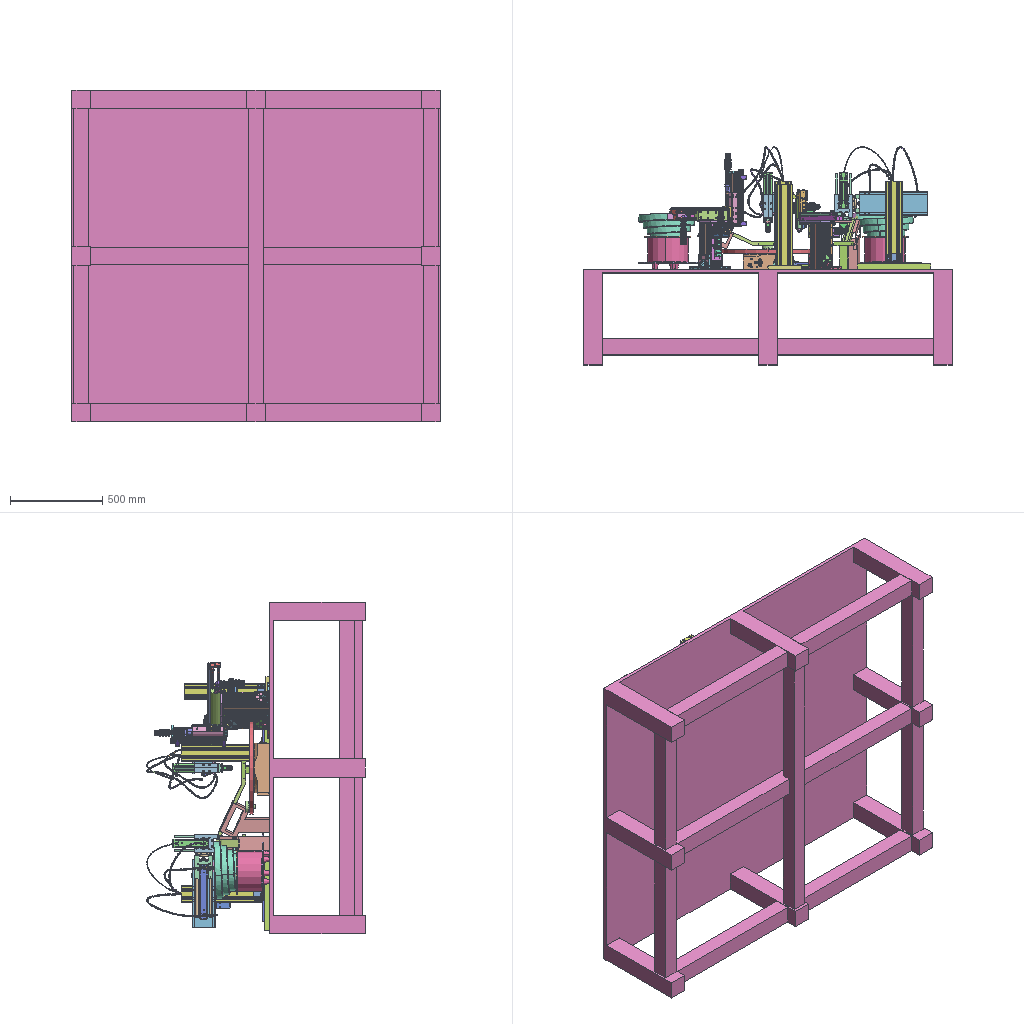Assembly | STEP file | 117 different items | 203 placed | box 2000 x 1188 x 1800 mm
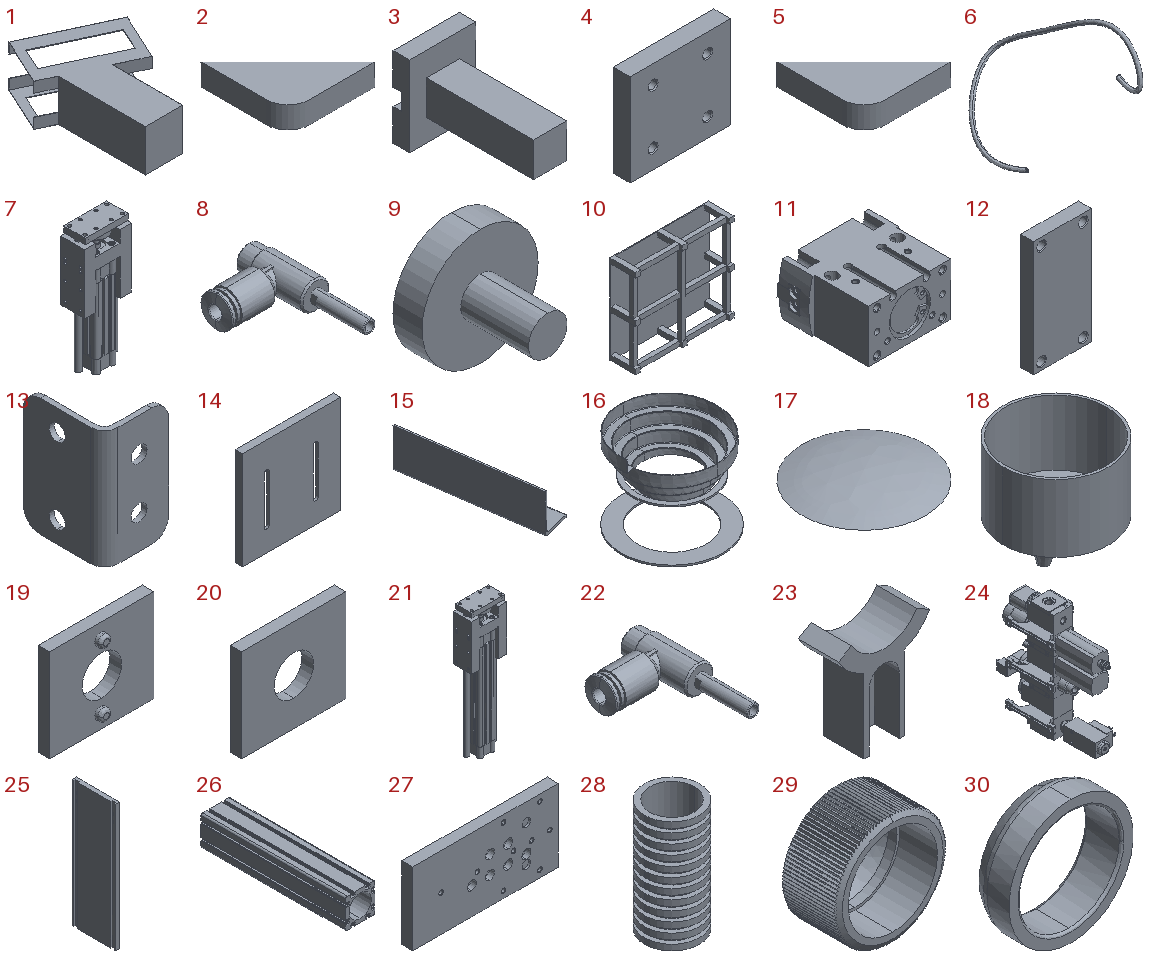Parts list (item | name | quantity | parent item | size | volume):
1 | Part3_4 | x2 | in BOBBIN PRESSING MACHINE | 195.46 x 270.819 x 80 mm | 83841 mm3
2 | Part9_5 | x6 | in BOBBIN PRESSING MACHINE | 20 x 20 x 5 mm | 973.175 mm3
3 | Part1_4 | x2 | in BOBBIN PRESSING MACHINE | 80 x 149.9 x 97 mm | 359263 mm3
4 | 555_4 | x2 | in BOBBIN PRESSING MACHINE | 60 x 10 x 54.9 mm | 31707 mm3
5 | Part8_5 | x6 | in BOBBIN PRESSING MACHINE | 20 x 20 x 5 mm | 973.175 mm3
6 | 332_4 | x2 | in BOBBIN PRESSING MACHINE | 176.185 x 279.344 x 194.737 mm | 23581 mm3
7 | 535411 DNCI-32-100-P-A-FENG-MS---(asm_0_)(control position cylinder 100)_5 | x2 | in BOBBIN PRESSING MACHINE | 97 x 50 x 265 mm | 701103 mm3
8 | 1_11 | x4 | in BOBBIN PRESSING MACHINE | 24.75 x 38 x 10 mm | 2280 mm3
9 | Part5_1 | x1 | in BOBBIN PRESSING MACHINE | 60 x 50 x 60 mm | 49793 mm3
10 | 223_4 | x1 | in BOBBIN PRESSING MACHINE | 2000 x 520 x 1800 mm | 184958483 mm3
11 | 535861 HGPT-20-A---(asm_0)_5 | x2 | in BOBBIN PRESSING MACHINE | 50 x 46 x 28 mm | 52148 mm3
12 | spacer_5 | x2 | in BOBBIN PRESSING MACHINE | 45 x 10 x 90 mm | 39110 mm3
13 | Part6_5 | x6 | in BOBBIN PRESSING MACHINE | 38 x 48 x 70 mm | 15736 mm3
14 | leg control03_5 | x2 | in BOBBIN PRESSING MACHINE | 400 x 30 x 400 mm | 2067797 mm3
15 | 444_4 | x2 | in bowel feeder_4 | 42.378 x 132.163 x 37.433 mm | 15585 mm3
16 | 222_4 | x2 | in bowel feeder_4 | 322.673 x 320.624 x 270.209 mm | 556791 mm3
17 | 111_4 | x2 | in bowel feeder_4 | 185.942 x 185.942 x 13.599 mm | 185950 mm3
18 | 333_4 | x2 | in bowel feeder_4 | 220 x 220 x 180 mm | 733955 mm3
19 | leg control01_5 | x2 | in BOBBIN PRESSING MACHINE | 180 x 30 x 160 mm | 509091 mm3
20 | Part10_5 | x1 | in BOBBIN PRESSING MACHINE | 180 x 20 x 160 mm | 503407 mm3
21 | 535411 DNCI-32-200-P-A-FENG-MS---(asm_0_)(control position cylinder with guide)_5 | x2 | in BOBBIN PRESSING MACHINE | 97 x 50 x 365 mm | 831843 mm3
22 | 1_10 | x4 | in BOBBIN PRESSING MACHINE | 24.75 x 38 x 10 mm | 2280 mm3
23 | jaw_5 | x4 | in BOBBIN PRESSING MACHINE | 18.187 x 8 x 20.75 mm | 920.185 mm3
24 | 542315 MSB4-1_4_C3J4M1D1A1F3-WP_5 | x1 | in BOBBIN PRESSING MACHINE | 85 x 221.2 x 244.7 mm | 1168039 mm3
25 | Part7_5 | x2 | in BOBBIN PRESSING MACHINE | 12 x 127 x 370 mm | 526068 mm3
26 | leg01_5 | x3 | in BOBBIN PRESSING MACHINE | 90 x 440 x 90 mm | 1490360 mm3
27 | 00684281_ADAPTERPLATTE_HMVY-1 | x1 | in 00539968_EZT_VERBINDUNGS-BS_HMVY-1 | 160 x 12 x 80 mm | 147813 mm3
28 | P0177567_EZT_SCHUTZSCHLAUCH_MKR-23-PG-21.1 | x1 | in HMI... | 28.5 x 28.5 x 58 mm | 8821 mm3
29 | 00649789_MUTTER_RAENDEL_MKRT-23-16.5 | x2 | in 00194321_EZT_SCHUTZSCHL.VERB_MKRT-23-16.5.1 | 35.488 x 19 x 35.5 mm | 6985 mm3
30 | 00399797_RING_ELASTOMER_MKRT-23-16.5 | x2 | in 00194321_EZT_SCHUTZSCHL.VERB_MKRT-23-16.5.1 | 26.7 x 8 x 26.7 mm | 1330 mm3
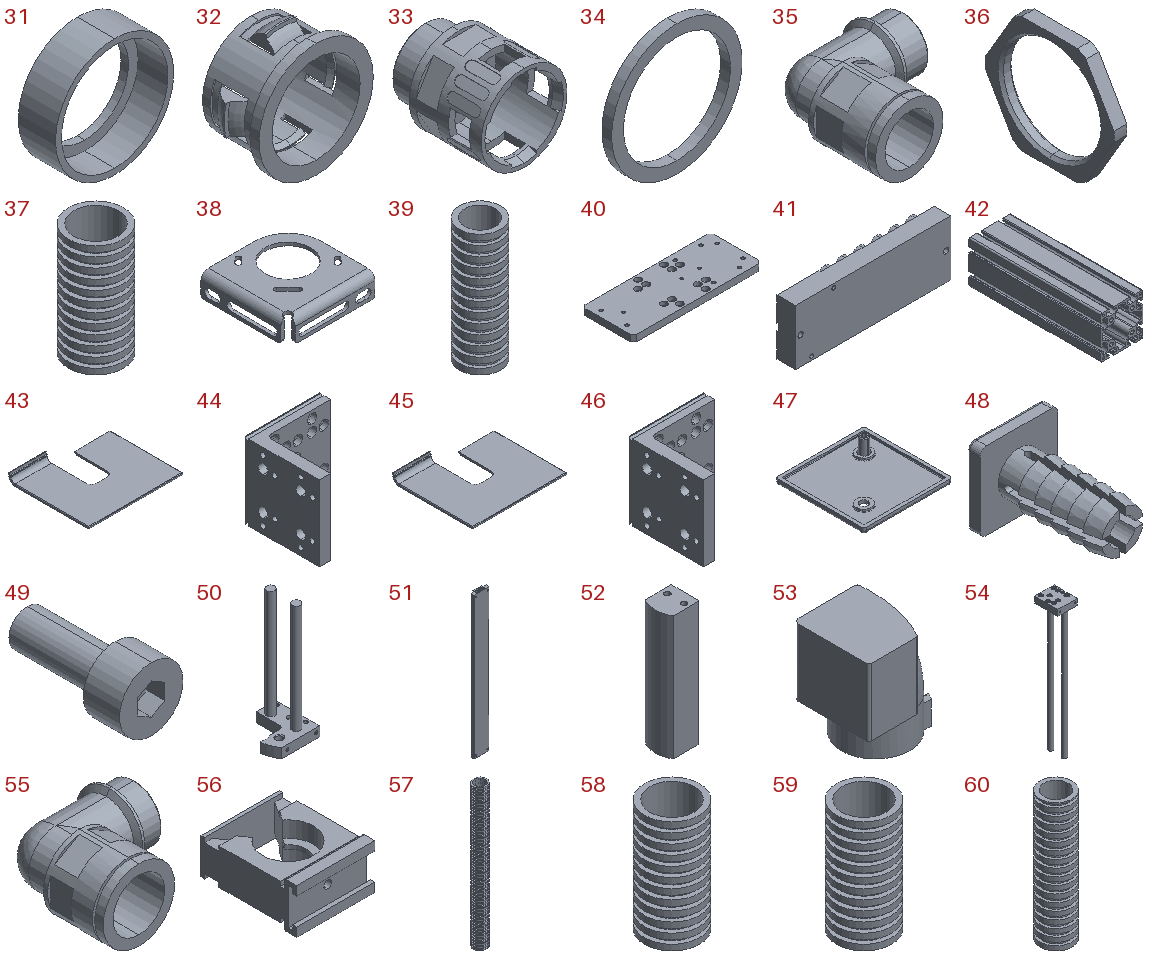31 | P2858E27_RING_DICHT | x4 | in 00177572_SCHUTZSCHL.VERS_MKRV-23-PG-21, 00177572_SCHUTZSCHL.VERS_MKRV-23-PG-21.1 | 31.6 x 10 x 31.6 mm | 1879 mm3
32 | P2858E25_EINSATZ_VERSCH. | x4 | in 00177572_SCHUTZSCHL.VERS_MKRV-23-PG-21, 00177572_SCHUTZSCHL.VERS_MKRV-23-PG-21.1 | 37 x 21 x 37 mm | 4042 mm3
33 | PN_0001 part X2_00DC_X0 throw | x4 | in 00177572_SCHUTZSCHL.VERS_MKRV-23-PG-21, 00177572_SCHUTZSCHL.VERS_MKRV-23-PG-21.1 | 37 x 43 x 37 mm | 10248 mm3
34 | 00649788_SCHEIBE_MKRT-23-16.5 | x2 | in 00194321_EZT_SCHUTZSCHL.VERB_MKRT-23-16.5.1 | 26.5 x 2 x 26.5 mm | 360.007 mm3
35 | 00177576_EZT_L-SCH.SCHL.VER._MKRL-16.5-PG-16 | x1 | in HMI... | 50.5 x 51.75 x 29.5 mm | 15308 mm3
36 | 00373407_MUTTER_M_PG_21_DIN_46320-MS | x3 | in 00177599_EZT_GEGENMUTTER_MKM-PG-21.1 | 3.5 x 35.5 x 32 mm | 1055 mm3
37 | P0177567_EZT_SCHUTZSCHLAUCH_MKR-23-PG-21.2 | x1 | in HMI... | 28.5 x 28.5 x 58 mm | 8821 mm3
38 | 00396465_ADAPTER_HMZAS-PG21 | x3 | in 00193124_EZT_ADAPTERPLATTE_HMZAS-PG-21.1 | 54.5 x 54.5 x 14 mm | 5523 mm3
39 | P0177566_EZT_SCHUTZSCHLAUCH_MKR-16.5-PG-16 | x1 | in HMI... | 21.2 x 21.2 x 63 mm | 7207 mm3
40 | 00398494_EZT_ADAPTERPLATTE_HMZV-1 | x1 | in HMZV-1 | 200 x 80 x 10 mm | 151646 mm3
41 | PRODUCT_NAME_42 | x1 | in 177670_MPV-E_A12-M8 | 126 x 19.5 x 45 mm | 83234 mm3
42 | 00175958_EZT_PROFILSAEULE_HMBS-80.80-250-.1 | x1 | in HMBS-1 | 80 x 250 x 80 mm | 517689 mm3
43 | 00371716_ABDECKKAPPE_HMB-....2 | x2 | in 00175967_EZT_VERBINDUNGS-BS_HMBV-ND.1 | 79.8 x 67.8 x 10.238 mm | 5792 mm3
44 | 00363089_WINKEL_HMB-..._1 | x1 | in 00175967_EZT_VERBINDUNGS-BS_HMBV-ND.1 | 80 x 80 x 80 mm | 130537 mm3
45 | 00371716_ABDECKKAPPE_HMB-....1 | x4 | in 00175951_EZT_GRUND-BS_HMBF-DB.1 | 79.8 x 67.8 x 10.238 mm | 5792 mm3
46 | 00363089_WINKEL_HMB-... | x2 | in 00175951_EZT_GRUND-BS_HMBF-DB.1 | 80 x 80 x 80 mm | 130537 mm3
47 | 00369089_KAPPE_ABDECK_IPM-AN-8-80X80 | x1 | in 00175965_ABDECKKAPPE_HMBSA-80_80.1 | 80 x 80 x 18 mm | 20980 mm3
48 | 00369095_STOPFEN_BEFEST._IPM-AB-8-SW | x1 | in 00175965_ABDECKKAPPE_HMBSA-80_80.1 | 12 x 18.5 x 12 mm | 599.689 mm3
49 | - | x4 | in 191182_HMPL-16-160-AI-VP-2A2 | 7 x 14 x 7 mm | 263.372 mm3
50 | - | x1 | in 191182_HMPL-16-160-AI-VP-2A2 | 54.828 x 55 x 147.5 mm | 42895 mm3
51 | P193368_BVP_HMPL_16_160 | x1 | in 191182_HMPL-16-160-AI-VP-2A2 | 45 x 14 x 426.6 mm | 169280 mm3
52 | - | x1 | in 191182_HMPL-16-160-AI-VP-2A2 | 56.5 x 53 x 234 mm | 627252 mm3
53 | P393261_cap_HMPL_16 | x1 | in 191182_HMPL-16-160-AI-VP-2A2 | 36.5 x 32.1 x 42.5 mm | 33239 mm3
54 | - | x1 | in 191182_HMPL-16-160-AI-VP-2A2 | 45 x 54 x 319 mm | 75910 mm3
55 | 00177577_EZT_L-SCH.SCHL.VER._MKRL-23-PG-21.1 | x1 | in HMI..._1 | 59.35 x 59.85 x 37 mm | 23850 mm3
56 | 00192290_EZT_KLEMMSCHELLE_MKRS-23-B.2 | x2 | in HMI..._1 | 43.5 x 53.5 x 25 mm | 24720 mm3
57 | P0177567_EZT_SCHUTZSCHLAUCH_MKR-23-PG-21.2_1 | x1 | in HMI..._1 | 28.5 x 28.5 x 303 mm | 45141 mm3
58 | P0177567_EZT_SCHUTZSCHLAUCH_MKR-23-PG-21.1_1 | x1 | in HMI..._1 | 28.5 x 28.5 x 58 mm | 8821 mm3
59 | P0177567_EZT_SCHUTZSCHLAUCH_MKR-23-PG-21.3 | x1 | in HMI..._1 | 28.5 x 28.5 x 58 mm | 8821 mm3
60 | P0177566_EZT_SCHUTZSCHLAUCH_MKR-16.5-PG-16_1 | x1 | in HMI..._1 | 21.2 x 21.2 x 85.851 mm | 9693 mm3
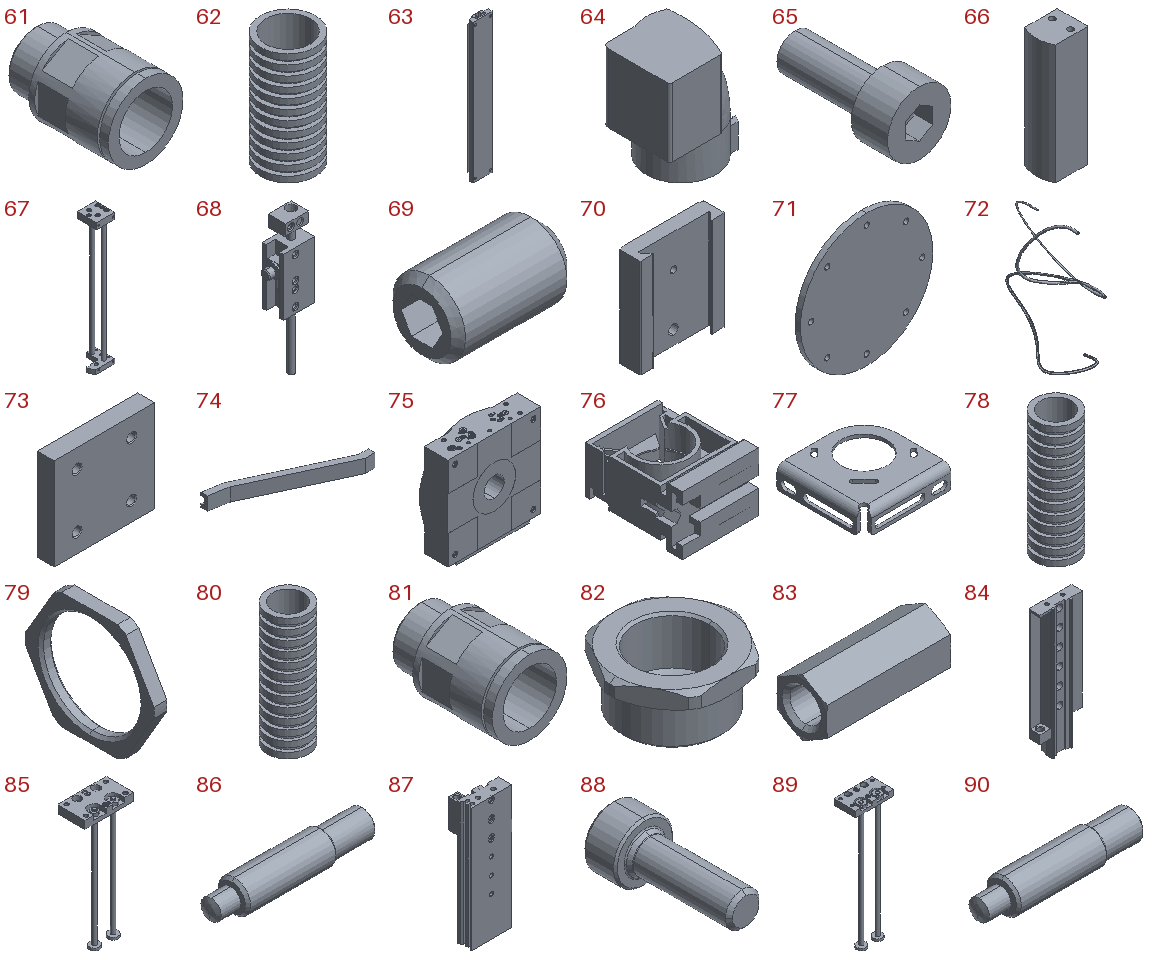61 | 00177571_EZT_SCHUTZSCHL.VERS_MKRV-16.5-PG-16.1 | x1 | in HMI..._1 | 29.5 x 43.5 x 29.5 mm | 11816 mm3
62 | P0177567_EZT_SCHUTZSCHLAUCH_MKR-23-PG-21.4 | x1 | in HMI..._1 | 28.5 x 28.5 x 58 mm | 8821 mm3
63 | P193372_BVP_HMPL_12_100 | x1 | in 191181_HMPL-12-100-AI-VP-KP-2A2 | 42 x 14 x 301.6 mm | 121442 mm3
64 | P393295_cap_HMPL_12 | x1 | in 191181_HMPL-12-100-AI-VP-KP-2A2 | 36.5 x 29.25 x 42.5 mm | 30561 mm3
65 | - | x4 | in 191181_HMPL-12-100-AI-VP-KP-2A2 | 7 x 14 x 7 mm | 263.372 mm3
66 | - | x1 | in 191181_HMPL-12-100-AI-VP-KP-2A2 | 51.8 x 44 x 171 mm | 352812 mm3
67 | - | x1 | in 191181_HMPL-12-100-AI-VP-KP-2A2 | 50.109 x 46 x 302 mm | 63535 mm3
68 | 00193112_FESTSTELLEINH._BKP-HMPL-12-80.100 | x1 | in 191181_HMPL-12-100-AI-VP-KP-2A2 | 52.1 x 29 x 190 mm | 85928 mm3
69 | 00245858_Gewinsestift | x2 | in 00193126_EZT_KLEMMELEMENT_HMPL-..-...2 | 10 x 6 x 6 mm | 243.919 mm3
70 | 00382584_HALTER_SCHWALB._HMPL-..-.. | x2 | in 00193126_EZT_KLEMMELEMENT_HMPL-..-...2 | 42 x 11 x 49 mm | 15212 mm3
71 | 113_4 | x1 | in BOBBIN PRESSING MACHINE | 500 x 20 x 500 mm | 3876725 mm3
72 | Part4_2 | x2 | in BOBBIN PRESSING MACHINE | - | -
73 | 442_4 | x2 | in BOBBIN PRESSING MACHINE | 60 x 10 x 54.9 mm | 31707 mm3
74 | Part2_4 | x2 | in BOBBIN PRESSING MACHINE | 368.104 x 160 x 40 mm | 215115 mm3
75 | 163302 DNC-32-200-P-A-V5---(asm_200)(index)_5 | x1 | in BOBBIN PRESSING MACHINE | 270 x 89 x 286.6 mm | 5960531 mm3
76 | 00192289_KLEMMSCHELLE_MKRS-16.5-B.1 | x1 | in HMI..._3 | 36.5 x 41.5 x 25 mm | 11692 mm3
77 | 00396465_ADAPTER_HMZAS-PG21_3 | x1 | in 00193124_EZT_ADAPTERPLATTE_HMZAS-PG-21.1_2 | 54.5 x 54.5 x 14 mm | 5523 mm3
78 | P0177566_EZT_SCHUTZSCHLAUCH_MKR-16.5-PG-16.2 | x1 | in HMI..._3 | 21.2 x 21.2 x 63 mm | 7207 mm3
79 | 00373407_MUTTER_M_PG_21_DIN_46320-MS_3 | x1 | in 00177599_EZT_GEGENMUTTER_MKM-PG-21.1_2 | 3.5 x 35.5 x 32 mm | 1055 mm3
80 | P0177566_EZT_SCHUTZSCHLAUCH_MKR-16.5-PG-16.1 | x1 | in HMI..._3 | 21.2 x 21.2 x 63 mm | 7207 mm3
81 | 00177571_EZT_SCHUTZSCHL.VERS_MKRV-16.5-PG-16.1_1 | x1 | in HMI..._3 | 29.5 x 43.5 x 29.5 mm | 11816 mm3
82 | 00193948_ADAPTERVERSCHR._MKA-PG-21-PG-16-KU.1 | x1 | in HMI..._3 | 35.5 x 32 x 16 mm | 5870 mm3
83 | - | x2 | in 197894_SLT-10-80-A-CC-B | 25 x 10 x 11.547 mm | 1346 mm3
84 | - | x1 | in 197894_SLT-10-80-A-CC-B | 50 x 15 x 153 mm | 64725 mm3
85 | - | x1 | in 197894_SLT-10-80-A-CC-B | 49.6 x 28 x 122 mm | 12171 mm3
86 | P649653_YSRT_5_5_C_1 | x2 | in 197894_SLT-10-80-A-CC-B | 38.3 x 8 x 8 mm | 1568 mm3
87 | - | x1 | in 197894_SLT-10-80-A-CC-B | 50 x 29.5 x 152 mm | 104448 mm3
88 | - | x2 | in 197894_SLT-10-80-A-CC-B | 7 x 16 x 7 mm | 280.848 mm3
89 | - | x1 | in 197901_SLT-16-150-A-CC-B | 65.6 x 38 x 218 mm | 33803 mm3
90 | P649654_YSRT_7_5_C | x2 | in 197901_SLT-16-150-A-CC-B | 44.8 x 10 x 10 mm | 2880 mm3
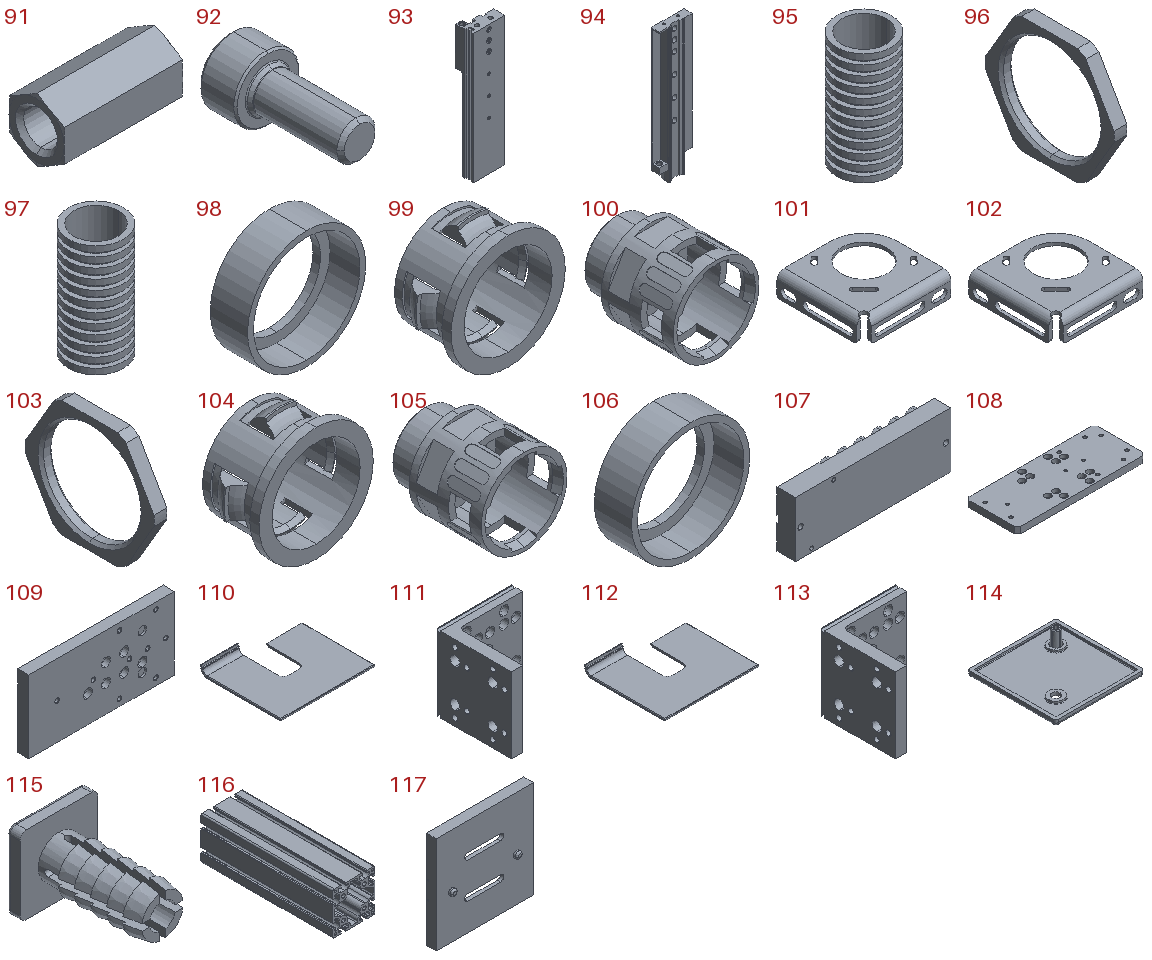91 | - | x2 | in 197901_SLT-16-150-A-CC-B | 28 x 13 x 15.011 mm | 2662 mm3
92 | - | x2 | in 197901_SLT-16-150-A-CC-B | 8.5 x 17 x 8.5 mm | 468.205 mm3
93 | - | x1 | in 197901_SLT-16-150-A-CC-B | 66 x 39.5 x 270 mm | 335701 mm3
94 | - | x1 | in 197901_SLT-16-150-A-CC-B | 66 x 18.5 x 270 mm | 203255 mm3
95 | P0177567_EZT_SCHUTZSCHLAUCH_MKR-23-PG-21.1_2 | x1 | in HMI..._2 | 28.5 x 28.5 x 58 mm | 8821 mm3
96 | 00373407_MUTTER_M_PG_21_DIN_46320-MS_2 | x1 | in 00177599_EZT_GEGENMUTTER_MKM-PG-21.1_1 | 3.5 x 35.5 x 32 mm | 1055 mm3
97 | P0177567_EZT_SCHUTZSCHLAUCH_MKR-23-PG-21.2_2 | x1 | in HMI..._2 | 28.5 x 28.5 x 58 mm | 8821 mm3
98 | P2858E27_RING_DICHT_2 | x1 | in 00177572_SCHUTZSCHL.VERS_MKRV-23-PG-21.2 | 31.6 x 10 x 31.6 mm | 1879 mm3
99 | P2858E25_EINSATZ_VERSCH._2 | x1 | in 00177572_SCHUTZSCHL.VERS_MKRV-23-PG-21.2 | 37 x 21 x 37 mm | 4042 mm3
100 | - | x1 | in 00177572_SCHUTZSCHL.VERS_MKRV-23-PG-21.2 | 37 x 43 x 37 mm | 10248 mm3
101 | 00396465_ADAPTER_HMZAS-PG21_1 | x1 | in 00193124_EZT_ADAPTERPLATTE_HMZAS-PG-21.1_1 | 54.5 x 54.5 x 14 mm | 5523 mm3
102 | 00396465_ADAPTER_HMZAS-PG21_2 | x1 | in 00193124_EZT_ADAPTERPLATTE_HMZAS-PG-21.2 | 54.5 x 54.5 x 14 mm | 5523 mm3
103 | 00373407_MUTTER_M_PG_21_DIN_46320-MS_1 | x1 | in 00177599_EZT_GEGENMUTTER_MKM-PG-21.2 | 3.5 x 35.5 x 32 mm | 1055 mm3
104 | P2858E25_EINSATZ_VERSCH._1 | x1 | in 00177572_SCHUTZSCHL.VERS_MKRV-23-PG-21.1_1 | 37 x 21 x 37 mm | 4042 mm3
105 | - | x1 | in 00177572_SCHUTZSCHL.VERS_MKRV-23-PG-21.1_1 | 37 x 43 x 37 mm | 10248 mm3
106 | P2858E27_RING_DICHT_1 | x1 | in 00177572_SCHUTZSCHL.VERS_MKRV-23-PG-21.1_1 | 31.6 x 10 x 31.6 mm | 1879 mm3
107 | PRODUCT_NAME_2 | x1 | in 177670 MPV-E_A12-M8.stp | 126 x 19.5 x 45 mm | 83234 mm3
108 | 00398494_EZT_ADAPTERPLATTE_HMZV-1_1 | x1 | in HMZV-1_1 | 200 x 80 x 10 mm | 151646 mm3
109 | 00684281_ADAPTERPLATTE_HMVY-1_1 | x1 | in 00539968_EZT_VERBINDUNGS-BS_HMVY-1_1 | 160 x 12 x 80 mm | 147813 mm3
110 | 00371716_ABDECKKAPPE_HMB-....1_1 | x4 | in 00175951_EZT_GRUND-BS_HMBF-DB.2 | 79.8 x 67.8 x 10.238 mm | 5792 mm3
111 | 00363089_WINKEL_HMB-..._2 | x2 | in 00175951_EZT_GRUND-BS_HMBF-DB.2 | 80 x 80 x 80 mm | 130537 mm3
112 | 00371716_ABDECKKAPPE_HMB-....2_1 | x2 | in 00175967_EZT_VERBINDUNGS-BS_HMBV-ND.1_1 | 79.8 x 67.8 x 10.238 mm | 5792 mm3
113 | 00363089_WINKEL_HMB-..._3 | x1 | in 00175967_EZT_VERBINDUNGS-BS_HMBV-ND.1_1 | 80 x 80 x 80 mm | 130537 mm3
114 | 00369089_KAPPE_ABDECK_IPM-AN-8-80X80_1 | x1 | in 00175965_ABDECKKAPPE_HMBSA-80_80.1_1 | 80 x 80 x 18 mm | 20980 mm3
115 | 00369095_STOPFEN_BEFEST._IPM-AB-8-SW_1 | x1 | in 00175965_ABDECKKAPPE_HMBSA-80_80.1_1 | 12 x 18.5 x 12 mm | 599.689 mm3
116 | 00175958_EZT_PROFILSAEULE_HMBS-80.80-250-.1_1 | x1 | in HMBS-1_1 | 80 x 250 x 80 mm | 517689 mm3
117 | leg control02_5 | x2 | in BOBBIN PRESSING MACHINE | 300 x 40 x 300 mm | 1254281 mm3
Placements (level | parent | child | x y z in mm | rotation matrix by rows), first 206 of 266 lines:
1 | BOBBIN PRESSING MACHINE | Part3_4 | 4.079 0.1 -57.688 | -0.1407 0 -0.9901 0 1 0 0.9901 0 -0.1407
1 | BOBBIN PRESSING MACHINE | Part9_5 | 172.7 -20.0 -269.933 | -1 0 0 0 1 0 0 0 -1
1 | BOBBIN PRESSING MACHINE | Part1_4 | 4.079 0.1 -57.688 | -0.1407 0 -0.9901 0 1 0 0.9901 0 -0.1407
1 | BOBBIN PRESSING MACHINE | 555_4 | -0.0 -0.0 -0.0 | 1 0 0 0 1 0 0 0 1
1 | BOBBIN PRESSING MACHINE | Part8_5 | 8.7 -31.841 1100.067 | 1 0 0 0 1 0 0 0 1
1 | BOBBIN PRESSING MACHINE | 332_4 | 114.93 -1.0 -11.041 | -0.9825 0 0.1862 0 1 0 -0.1862 0 -0.9825
1 | BOBBIN PRESSING MACHINE | 535411 DNCI-32-100-P-A-FENG-MS---(asm_0_)(control position cylinder 100)_5 | 0.0 301.0 -410.0 | 0 -1 0 0 0 -1 1 0 0
1 | BOBBIN PRESSING MACHINE | 1_11 | 800.0 328.0 -33.7 | 0 0 -1 1 0 0 0 -1 -0
1 | BOBBIN PRESSING MACHINE | Part3_4 | -0.0 -0.0 -0.0 | 1 0 0 0 1 0 0 0 1
1 | BOBBIN PRESSING MACHINE | Part5_1 | -0.0 -0.0 -0.0 | 1 0 0 0 1 0 0 0 1
1 | BOBBIN PRESSING MACHINE | 223_4 | -0.0 -30.0 -0.0 | 1 0 0 0 1 0 0 0 1
1 | BOBBIN PRESSING MACHINE | 535861 HGPT-20-A---(asm_0)_5 | -0.0 224.0 -410.0 | 0 0 -1 0 -1 0 -1 0 -0
1 | BOBBIN PRESSING MACHINE | spacer_5 | -0.0 -0.0 -0.0 | 1 0 0 0 1 0 0 0 1
1 | BOBBIN PRESSING MACHINE | Part9_5 | 164.0 -0.0 -1370.0 | -1 0 0 0 1 0 0 0 -1
1 | BOBBIN PRESSING MACHINE | Part6_5 | 1370.0 8.1 164.0 | 0 0 1 0 1 0 -1 0 0
1 | BOBBIN PRESSING MACHINE | Part6_5 | -0.0 8.1 -0.0 | 0 0 -1 0 1 0 1 0 -0
1 | BOBBIN PRESSING MACHINE | leg control03_5 | -0.0 -0.0 -0.0 | 0 0 -1 0 1 0 1 0 -0
1 | BOBBIN PRESSING MACHINE | bowel feeder_4 | 635.899 110.1 -517.537 | 0.9612 0.2758 0 0 0 1 0.2758 -0.9612 0
2 | bowel feeder_4 | 444_4 | -0.0 -0.0 -0.0 | 1 0 0 0 1 0 0 0 1
2 | bowel feeder_4 | 222_4 | -0.0 -0.0 -0.0 | 1 0 0 0 1 0 0 0 1
2 | bowel feeder_4 | 111_4 | -0.0 -0.0 43.623 | 1 0 0 0 1 0 0 0 1
2 | bowel feeder_4 | 333_4 | -0.0 -0.0 -0.0 | 1 0 0 0 1 0 0 0 1
1 | BOBBIN PRESSING MACHINE | 1_11 | 410.0 320.5 -33.7 | -0.01784 0 0.9998 -0.9998 0 -0.01784 0 -1 -0
1 | BOBBIN PRESSING MACHINE | spacer_5 | -0.0 -0.0 -0.0 | 0 0 -1 0 1 0 1 0 -0
1 | BOBBIN PRESSING MACHINE | leg control01_5 | -0.0 -0.0 -0.0 | 0 0 -1 0 1 0 1 0 -0
1 | BOBBIN PRESSING MACHINE | Part10_5 | -0.0 -0.0 -244.308 | 1 0 0 0 1 0 0 0 1
1 | BOBBIN PRESSING MACHINE | bowel feeder_4 | -544.173 110.1 -560.833 | 0.1378 -0.9905 0 0 0 1 -0.9905 -0.1378 0
2 | bowel feeder_4 | 444_4 | -0.0 -0.0 -0.0 | 1 0 0 0 1 0 0 0 1
2 | bowel feeder_4 | 222_4 | -0.0 -0.0 -0.0 | 1 0 0 0 1 0 0 0 1
2 | bowel feeder_4 | 111_4 | -0.0 -0.0 43.623 | 1 0 0 0 1 0 0 0 1
2 | bowel feeder_4 | 333_4 | -0.0 -0.0 -0.0 | 1 0 0 0 1 0 0 0 1
1 | BOBBIN PRESSING MACHINE | 1_11 | -33.7 328.0 -800.0 | 0 -1 0 1 0 0 0 0 1
1 | BOBBIN PRESSING MACHINE | leg control03_5 | -0.0 -0.0 -0.0 | 1 0 0 0 1 0 0 0 1
1 | BOBBIN PRESSING MACHINE | Part6_5 | -0.0 8.1 -0.0 | 1 0 0 0 1 0 0 0 1
1 | BOBBIN PRESSING MACHINE | 535411 DNCI-32-200-P-A-FENG-MS---(asm_0_)(control position cylinder with guide)_5 | 525.5 328.0 0.0 | 0 0 -1 1 0 0 0 -1 -0
1 | BOBBIN PRESSING MACHINE | Part6_5 | 172.7 -11.9 -269.933 | -1 0 0 0 1 0 0 0 -1
1 | BOBBIN PRESSING MACHINE | Part8_5 | 0.0 -11.841 -0.0 | 1 0 0 0 1 0 0 0 1
1 | BOBBIN PRESSING MACHINE | 1_10 | 545.0 328.0 -33.7 | 0 0 -1 1 0 0 0 -1 -0
1 | BOBBIN PRESSING MACHINE | 535411 DNCI-32-200-P-A-FENG-MS---(asm_0_)(control position cylinder with guide)_5 | 0.0 328.0 -525.5 | 0 -1 0 1 0 0 0 0 1
1 | BOBBIN PRESSING MACHINE | Part8_5 | 1370.0 -11.841 164.0 | 0 0 1 0 1 0 -1 0 0
1 | BOBBIN PRESSING MACHINE | 535861 HGPT-20-A---(asm_0)_5 | 410.0 224.0 -0.0 | 1 0 0 0 -1 0 0 0 -1
1 | BOBBIN PRESSING MACHINE | jaw_5 | 820.0 -0.0 0.0 | 0 0 1 0 1 0 -1 0 0
1 | BOBBIN PRESSING MACHINE | 542315 MSB4-1_4_C3J4M1D1A1F3-WP_5 | 170.5 304.931 -524.435 | 1 0 0 0 1 0 0 0 1
1 | BOBBIN PRESSING MACHINE | Part7_5 | -0.0 -0.0 -0.0 | 0 0 -1 0 1 0 1 0 -0
1 | BOBBIN PRESSING MACHINE | leg01_5 | 8.7 -20.0 1100.067 | 1 0 0 0 1 0 0 0 1
1 | BOBBIN PRESSING MACHINE | 1_10 | -33.7 328.0 -545.0 | 0 -1 0 1 0 0 0 0 1
1 | BOBBIN PRESSING MACHINE | Part9_5 | -0.0 -0.0 -0.0 | 1 0 0 0 1 0 0 0 1
1 | BOBBIN PRESSING MACHINE | Part8_5 | 164.0 -11.841 -1370.0 | -1 0 0 0 1 0 0 0 -1
1 | BOBBIN PRESSING MACHINE | 332_4 | 49.106 -0.0 -122.369 | -0.04642 0 -0.9989 0 1 0 0.9989 0 -0.04642
1 | BOBBIN PRESSING MACHINE | Part9_5 | 1370.0 -0.0 164.0 | 0 0 1 0 1 0 -1 0 0
1 | BOBBIN PRESSING MACHINE | Part8_5 | 172.7 -31.841 -269.933 | -1 0 0 0 1 0 0 0 -1
1 | BOBBIN PRESSING MACHINE | 542973_DHSP_DKI_HMPL16_160-HMPL12_100 | -316.814 -29.9 290.79 | -0.6788 0.7343 0 0 0 1 0.7343 0.6788 0
2 | 542973_DHSP_DKI_HMPL16_160-HMPL12_100 | HMSSY-PP-HMPL-1_HMPL-16_V002 | -600.0 -0.0 -0.0 | 1 0 0 0 1 0 0 0 1
3 | HMSSY-PP-HMPL-1_HMPL-16_V002 | HMBSY-HMPL-1 | -0.0 0.0 -0.0 | 1 0 0 0 1 0 0 0 1
4 | HMBSY-HMPL-1 | 00539968_EZT_VERBINDUNGS-BS_HMVY-1 | 1097.0 520.0 302.2 | -1 0 0 0 0 1 0 1 -0
5 | 00539968_EZT_VERBINDUNGS-BS_HMVY-1 | 00684281_ADAPTERPLATTE_HMVY-1 | -15.0 -5.0 -0.0 | 1 0 0 0 1 0 0 0 1
4 | HMBSY-HMPL-1 | HMI... | -0.0 -0.0 -0.0 | 1 0 0 0 1 0 0 0 1
5 | HMI... | P0177567_EZT_SCHUTZSCHLAUCH_MKR-23-PG-21.1 | 1161.16 163.5 319.0 | 0 0 -1 0 -1 0 -1 0 0
5 | HMI... | 00194321_EZT_SCHUTZSCHL.VERB_MKRT-23-16.5.1 | 820.75 10.0 167.02 | 1 0 0 0 0 -1 0 1 0
6 | 00194321_EZT_SCHUTZSCHL.VERB_MKRT-23-16.5.1 | 00649789_MUTTER_RAENDEL_MKRT-23-16.5 | -0.0 1.0 0.0 | 1 0 0 0 1 0 0 0 1
6 | 00194321_EZT_SCHUTZSCHL.VERB_MKRT-23-16.5.1 | 00399797_RING_ELASTOMER_MKRT-23-16.5 | -0.0 1.0 0.0 | 1 0 0 0 1 0 0 0 1
6 | 00194321_EZT_SCHUTZSCHL.VERB_MKRT-23-16.5.1 | 00177572_SCHUTZSCHL.VERS_MKRV-23-PG-21 | 0.0 -0.0 950.0 | 1 0 0 0 1 0 0 0 1
7 | 00177572_SCHUTZSCHL.VERS_MKRV-23-PG-21 | P2858E27_RING_DICHT | -0.0 0.0 -950.0 | 1 0 0 0 1 0 0 0 1
7 | 00177572_SCHUTZSCHL.VERS_MKRV-23-PG-21 | P2858E25_EINSATZ_VERSCH. | -0.0 -4.0 -950.0 | 1 0 0 0 1 0 0 0 1
7 | 00177572_SCHUTZSCHL.VERS_MKRV-23-PG-21 | PN_0001 part X2_00DC_X0 throw | -0.0 0.0 -950.0 | 1 0 0 0 1 0 0 0 1
6 | 00194321_EZT_SCHUTZSCHL.VERB_MKRT-23-16.5.1 | 00649788_SCHEIBE_MKRT-23-16.5 | -0.0 -0.0 -0.0 | 1 0 0 0 1 0 0 0 1
5 | HMI... | 00177576_EZT_L-SCH.SCHL.VER._MKRL-16.5-PG-16 | 820.75 10.0 245.35 | -1 0 0 0 0 1 0 1 -0
5 | HMI... | 00177599_EZT_GEGENMUTTER_MKM-PG-21.1 | 356.0 692.523 346.423 | 0 0 1 0.5 0.866 0 -0.866 0.5 -0
6 | 00177599_EZT_GEGENMUTTER_MKM-PG-21.1 | 00373407_MUTTER_M_PG_21_DIN_46320-MS | -165.5 -561.5 321.25 | 0 0 -1 0 -1 0 -1 0 0
5 | HMI... | P0177567_EZT_SCHUTZSCHLAUCH_MKR-23-PG-21.2 | 930.75 50.0 -283.88 | -1 0 0 0 -1 0 0 0 1
5 | HMI... | 00193124_EZT_ADAPTERPLATTE_HMZAS-PG-21.1 | 680.0 68.0 178.5 | 0 0 -1 -1 0 0 0 1 0
6 | 00193124_EZT_ADAPTERPLATTE_HMZAS-PG-21.1 | 00396465_ADAPTER_HMZAS-PG21 | -15.0 18.0 -8.25 | -1 0 0 0 1 0 0 0 -1
5 | HMI... | P0177566_EZT_SCHUTZSCHLAUCH_MKR-16.5-PG-16 | 710.75 50.0 716.92 | 1 0 0 0 -1 0 0 0 -1
5 | HMI... | 00177572_SCHUTZSCHL.VERS_MKRV-23-PG-21.1 | 710.26 123.5 209.0 | 0 -1 0 0 0 -1 1 0 0
6 | 00177572_SCHUTZSCHL.VERS_MKRV-23-PG-21.1 | P2858E27_RING_DICHT | -0.0 -0.0 -0.0 | 1 0 0 0 1 0 0 0 1
6 | 00177572_SCHUTZSCHL.VERS_MKRV-23-PG-21.1 | PN_0001 part X2_00DC_X0 throw | -0.0 -0.0 -0.0 | 1 0 0 0 1 0 0 0 1
6 | 00177572_SCHUTZSCHL.VERS_MKRV-23-PG-21.1 | P2858E25_EINSATZ_VERSCH. | -0.0 -4.0 -0.0 | 1 0 0 0 1 0 0 0 1
4 | HMBSY-HMPL-1 | HMZV-1 | 600.0 900.0 0.0 | 1 0 0 0 1 0 0 0 1
5 | HMZV-1 | 00398494_EZT_ADAPTERPLATTE_HMZV-1 | -0.0 -810.0 50.0 | 0 1 0 0 0 1 1 0 -0
5 | HMZV-1 | 177670_MPV-E_A12-M8 | 40.0 -810.0 71.0 | 0 0 -1 0 1 0 1 0 0
6 | 177670_MPV-E_A12-M8 | PRODUCT_NAME_42 | 0.0 -0.0 -0.0 | 1 0 0 0 1 0 0 0 1
4 | HMBSY-HMPL-1 | HMBS-1 | 110.0 47.0 250.2 | 1 0 0 0 0 1 0 -1 -0
5 | HMBS-1 | 00175958_EZT_PROFILSAEULE_HMBS-80.80-250-.1 | 530.0 0.2 -7.0 | 1 0 0 0 1 0 0 0 1
5 | HMBS-1 | 00175967_EZT_VERBINDUNGS-BS_HMBV-ND.1 | 490.0 -4.8 -7.0 | -1 0 0 0 -1 0 0 0 1
6 | 00175967_EZT_VERBINDUNGS-BS_HMBV-ND.1 | 00371716_ABDECKKAPPE_HMB-....2 | 79.8 -13.5 -39.9 | 0 -1 0 0 0 -1 1 0 0
6 | 00175967_EZT_VERBINDUNGS-BS_HMBV-ND.1 | 00371716_ABDECKKAPPE_HMB-....2 | 13.5 -79.8 39.9 | 0 0 1 0 1 0 -1 0 0
6 | 00175967_EZT_VERBINDUNGS-BS_HMBV-ND.1 | 00363089_WINKEL_HMB-..._1 | -0.0 -0.0 -0.0 | 1 0 0 0 1 0 0 0 1
5 | HMBS-1 | 00175951_EZT_GRUND-BS_HMBF-DB.1 | 490.0 250.2 -7.0 | -1 0 0 0 1 0 0 0 -1
6 | 00175951_EZT_GRUND-BS_HMBF-DB.1 | 00371716_ABDECKKAPPE_HMB-....1 | 13.5 -79.8 39.9 | 0 0 1 0 1 0 -1 0 0
6 | 00175951_EZT_GRUND-BS_HMBF-DB.1 | 00371716_ABDECKKAPPE_HMB-....1 | 79.8 -13.5 -39.9 | 0 -1 0 0 0 -1 1 0 0
6 | 00175951_EZT_GRUND-BS_HMBF-DB.1 | 00363089_WINKEL_HMB-... | -0.0 -0.0 -0.0 | 1 0 0 0 1 0 0 0 1
5 | HMBS-1 | 00175951_EZT_GRUND-BS_HMBF-DB.1 | 570.0 250.2 -7.0 | 1 0 0 0 1 0 0 0 1
6 | 00175951_EZT_GRUND-BS_HMBF-DB.1 | 00371716_ABDECKKAPPE_HMB-....1 | 13.5 -79.8 39.9 | 0 0 1 0 1 0 -1 0 0
6 | 00175951_EZT_GRUND-BS_HMBF-DB.1 | 00371716_ABDECKKAPPE_HMB-....1 | 79.8 -13.5 -39.9 | 0 -1 0 0 0 -1 1 0 0
6 | 00175951_EZT_GRUND-BS_HMBF-DB.1 | 00363089_WINKEL_HMB-... | -0.0 -0.0 -0.0 | 1 0 0 0 1 0 0 0 1
5 | HMBS-1 | 00175965_ABDECKKAPPE_HMBSA-80_80.1 | 430.0 -238.9 -279 | 1 0 0 0 -1 0 0 0 -1
6 | 00175965_ABDECKKAPPE_HMBSA-80_80.1 | 00369089_KAPPE_ABDECK_IPM-AN-8-80X80 | 60.0 -239.1 -232 | 0 1 0 0 0 -1 -1 0 -0
6 | 00175965_ABDECKKAPPE_HMBSA-80_80.1 | 00369095_STOPFEN_BEFEST._IPM-AB-8-SW | 80.0 -252.1 -252 | 0 0 1 0 1 0 -1 0 0
3 | HMSSY-PP-HMPL-1_HMPL-16_V002 | antrieb | -0.0 0.0 -0.0 | 1 0 0 0 1 0 0 0 1
4 | antrieb | 191182_HMPL-16-160-AI-VP-2A2 | 520.5 59.0 322.0 | 0 0 -1 1 0 0 0 -1 0
5 | 191182_HMPL-16-160-AI-VP-2A2 | subassembly 2 | -40.5 -4.9 10.5 | 1 0 0 0 1 0 0 0 1
5 | 191182_HMPL-16-160-AI-VP-2A2 | subassembly 3 | -0.0 0.0 -0.0 | 1 0 0 0 1 0 0 0 1
5 | 191182_HMPL-16-160-AI-VP-2A2 | P193368_BVP_HMPL_16_160 | -22.5 0.0 17.3 | 1 0 0 0 -1 0 0 0 -1
5 | 191182_HMPL-16-160-AI-VP-2A2 | subassembly 4 | -0.0 0.0 -0.0 | 1 0 0 0 1 0 0 0 1
5 | 191182_HMPL-16-160-AI-VP-2A2 | subassembly 2 | -40.5 -4.9 -402.5 | 1 0 0 0 1 0 0 0 1
5 | 191182_HMPL-16-160-AI-VP-2A2 | subassembly 2 | -4.5 -4.9 -402.5 | 1 0 0 0 1 0 0 0 1
5 | 191182_HMPL-16-160-AI-VP-2A2 | P393261_cap_HMPL_16 | -29.5 55.0 -234.0 | -1 0 0 0 -1 0 0 0 1
5 | 191182_HMPL-16-160-AI-VP-2A2 | subassembly 5 | -0.0 0.0 -0.0 | 1 0 0 0 1 0 0 0 1
5 | 191182_HMPL-16-160-AI-VP-2A2 | subassembly 2 | -4.5 -4.9 10.5 | 1 0 0 0 1 0 0 0 1
2 | 542973_DHSP_DKI_HMPL16_160-HMPL12_100 | HMSSZ-PP-HMPL-1_HMPL-12_V002 | -600.0 -0.0 -0.0 | 1 0 0 0 1 0 0 0 1
3 | HMSSZ-PP-HMPL-1_HMPL-12_V002 | HMBSZ-HMPL-1 | -0.0 0.0 -0.0 | 1 0 0 0 1 0 0 0 1
4 | HMBSZ-HMPL-1 | HMI..._1 | -0.0 -0.0 -0.0 | 1 0 0 0 1 0 0 0 1
5 | HMI..._1 | 00177577_EZT_L-SCH.SCHL.VER._MKRL-23-PG-21.1 | 571.89 123.5 251.85 | 1 0 0 0 0 1 0 -1 -0
5 | HMI..._1 | 00192290_EZT_KLEMMSCHELLE_MKRS-23-B.2 | 381.25 26.999 500.15 | -3e-05 -1 0 1 -3e-05 0 0 0 1
5 | HMI..._1 | P0177567_EZT_SCHUTZSCHLAUCH_MKR-23-PG-21.2_1 | 271.249 66.996 889.45 | 1 3e-05 0 3e-05 -1 0 0 0 -1
5 | HMI..._1 | P0177567_EZT_SCHUTZSCHLAUCH_MKR-23-PG-21.1_1 | 350.25 44.5 1046.451 | 1 0 0 0 -1 0 0 0 -1
5 | HMI..._1 | 00193124_EZT_ADAPTERPLATTE_HMZAS-PG-21.1 | 588.5 93.0 250.0 | -1 0 0 0 1 0 0 0 -1
6 | 00193124_EZT_ADAPTERPLATTE_HMZAS-PG-21.1 | 00396465_ADAPTER_HMZAS-PG21 | -15.0 18.0 -8.25 | -1 0 0 0 1 0 0 0 -1
5 | HMI..._1 | P0177567_EZT_SCHUTZSCHLAUCH_MKR-23-PG-21.3 | 534.0 163.5 731.15 | 1 0 0 0 -1 0 0 0 -1
5 | HMI..._1 | 00193124_EZT_ADAPTERPLATTE_HMZAS-PG-21.1 | 600.0 93.0 153.5 | 0 0 1 0 1 0 -1 0 -0
6 | 00193124_EZT_ADAPTERPLATTE_HMZAS-PG-21.1 | 00396465_ADAPTER_HMZAS-PG21 | -15.0 18.0 -8.25 | -1 0 0 0 1 0 0 0 -1
5 | HMI..._1 | 00177599_EZT_GEGENMUTTER_MKM-PG-21.1 | 506.577 692.523 -74.0 | 0.866 -0.5 0 0.5 0.866 0 0 0 1
6 | 00177599_EZT_GEGENMUTTER_MKM-PG-21.1 | 00373407_MUTTER_M_PG_21_DIN_46320-MS | -165.5 -561.5 321.25 | 0 0 -1 0 -1 0 -1 0 0
5 | HMI..._1 | P0177566_EZT_SCHUTZSCHLAUCH_MKR-16.5-PG-16_1 | 350.25 -35.5 45.8 | 1 0 0 0 1 0 0 0 1
5 | HMI..._1 | 00177599_EZT_GEGENMUTTER_MKM-PG-21.1 | 924.0 692.523 71.577 | 0 0 -1 0.5 0.866 0 0.866 -0.5 -0
6 | 00177599_EZT_GEGENMUTTER_MKM-PG-21.1 | 00373407_MUTTER_M_PG_21_DIN_46320-MS | -165.5 -561.5 321.25 | 0 0 -1 0 -1 0 -1 0 0
5 | HMI..._1 | 00177571_EZT_SCHUTZSCHL.VERS_MKRV-16.5-PG-16.1 | 460.25 4.5 493.8 | 1 0 0 0 0 1 0 -1 -0
5 | HMI..._1 | P0177567_EZT_SCHUTZSCHLAUCH_MKR-23-PG-21.4 | 461.89 163.5 699.29 | 1 0 0 0 -1 0 0 0 -1
5 | HMI..._1 | 00192290_EZT_KLEMMSCHELLE_MKRS-23-B.2 | 381.25 26.999 247.55 | -3e-05 -1 0 1 -3e-05 0 0 0 1
5 | HMI..._1 | 00194321_EZT_SCHUTZSCHL.VERB_MKRT-23-16.5.1 | 460.25 4.5 595.551 | 1 0 0 0 0 1 0 -1 -0
6 | 00194321_EZT_SCHUTZSCHL.VERB_MKRT-23-16.5.1 | 00649789_MUTTER_RAENDEL_MKRT-23-16.5 | -0.0 1.0 0.0 | 1 0 0 0 1 0 0 0 1
6 | 00194321_EZT_SCHUTZSCHL.VERB_MKRT-23-16.5.1 | 00399797_RING_ELASTOMER_MKRT-23-16.5 | -0.0 1.0 0.0 | 1 0 0 0 1 0 0 0 1
6 | 00194321_EZT_SCHUTZSCHL.VERB_MKRT-23-16.5.1 | 00177572_SCHUTZSCHL.VERS_MKRV-23-PG-21 | 0.0 -0.0 950.0 | 1 0 0 0 1 0 0 0 1
7 | 00177572_SCHUTZSCHL.VERS_MKRV-23-PG-21 | P2858E27_RING_DICHT | -0.0 0.0 -950.0 | 1 0 0 0 1 0 0 0 1
7 | 00177572_SCHUTZSCHL.VERS_MKRV-23-PG-21 | P2858E25_EINSATZ_VERSCH. | -0.0 -4.0 -950.0 | 1 0 0 0 1 0 0 0 1
7 | 00177572_SCHUTZSCHL.VERS_MKRV-23-PG-21 | PN_0001 part X2_00DC_X0 throw | -0.0 0.0 -950.0 | 1 0 0 0 1 0 0 0 1
6 | 00194321_EZT_SCHUTZSCHL.VERB_MKRT-23-16.5.1 | 00649788_SCHEIBE_MKRT-23-16.5 | -0.0 -0.0 -0.0 | 1 0 0 0 1 0 0 0 1
5 | HMI..._1 | 00177572_SCHUTZSCHL.VERS_MKRV-23-PG-21.1 | 644.0 123.5 280.25 | -1 0 0 0 0 -1 0 -1 0
6 | 00177572_SCHUTZSCHL.VERS_MKRV-23-PG-21.1 | P2858E27_RING_DICHT | -0.0 -0.0 -0.0 | 1 0 0 0 1 0 0 0 1
6 | 00177572_SCHUTZSCHL.VERS_MKRV-23-PG-21.1 | PN_0001 part X2_00DC_X0 throw | -0.0 -0.0 -0.0 | 1 0 0 0 1 0 0 0 1
6 | 00177572_SCHUTZSCHL.VERS_MKRV-23-PG-21.1 | P2858E25_EINSATZ_VERSCH. | -0.0 -4.0 -0.0 | 1 0 0 0 1 0 0 0 1
3 | HMSSZ-PP-HMPL-1_HMPL-12_V002 | antrieb_1 | -0.0 0.0 -0.0 | 1 0 0 0 1 0 0 0 1
4 | antrieb_1 | 191181_HMPL-12-100-AI-VP-KP-2A2 | 429.0 48.0 248.8 | 0 1 0 1 0 0 0 0 -1
5 | 191181_HMPL-12-100-AI-VP-KP-2A2 | P193372_BVP_HMPL_12_100 | -21.0 -0.0 17.3 | 1 0 0 0 -1 0 0 0 -1
5 | 191181_HMPL-12-100-AI-VP-KP-2A2 | P393295_cap_HMPL_12 | -24.0 46.0 -171.0 | -1 0 0 0 -1 0 0 0 1
5 | 191181_HMPL-12-100-AI-VP-KP-2A2 | subassembly 6 | -4.75 -4.9 10.5 | 1 0 0 0 1 0 0 0 1
5 | 191181_HMPL-12-100-AI-VP-KP-2A2 | subassembly 6 | -37.25 -4.9 10.5 | 1 0 0 0 1 0 0 0 1
5 | 191181_HMPL-12-100-AI-VP-KP-2A2 | subassembly 7 | -0.0 -0.0 0.0 | 1 0 0 0 1 0 0 0 1
5 | 191181_HMPL-12-100-AI-VP-KP-2A2 | subassembly 8 | -0.0 -0.0 0.0 | 1 0 0 0 1 0 0 0 1
5 | 191181_HMPL-12-100-AI-VP-KP-2A2 | 00193112_FESTSTELLEINH._BKP-HMPL-12-80.100 | -39.5 45.0 17.3 | 1 0 0 0 1 0 0 0 1
5 | 191181_HMPL-12-100-AI-VP-KP-2A2 | subassembly 6 | -37.25 -4.9 -277.5 | 1 0 0 0 1 0 0 0 1
5 | 191181_HMPL-12-100-AI-VP-KP-2A2 | subassembly 6 | -4.75 -4.9 -277.5 | 1 0 0 0 1 0 0 0 1
4 | antrieb_1 | ZUB | -0.0 -0.0 -0.0 | 1 0 0 0 1 0 0 0 1
5 | ZUB | 00193126_EZT_KLEMMELEMENT_HMPL-..-...2 | 552.958 -33.895 519.85 | 3e-05 -1 0 -1 -3e-05 0 0 0 -1
6 | 00193126_EZT_KLEMMELEMENT_HMPL-..-...2 | 00245858_Gewinsestift | -60.899 146.957 -6.25 | 0 1 0 -1 0 0 0 0 1
6 | 00193126_EZT_KLEMMELEMENT_HMPL-..-...2 | 00382584_HALTER_SCHWALB._HMPL-..-.. | -0.0 -0.0 1.75 | 1 0 0 0 1 0 0 0 1
5 | ZUB | 00193126_EZT_KLEMMELEMENT_HMPL-..-...2 | 552.958 -33.895 267.25 | 3e-05 -1 0 -1 -3e-05 0 0 0 -1
6 | 00193126_EZT_KLEMMELEMENT_HMPL-..-...2 | 00245858_Gewinsestift | -60.899 146.957 -6.25 | 0 1 0 -1 0 0 0 0 1
6 | 00193126_EZT_KLEMMELEMENT_HMPL-..-...2 | 00382584_HALTER_SCHWALB._HMPL-..-.. | -0.0 -0.0 1.75 | 1 0 0 0 1 0 0 0 1
1 | BOBBIN PRESSING MACHINE | 113_4 | -0.0 -30.0 -0.0 | 1 0 0 0 1 0 0 0 1
1 | BOBBIN PRESSING MACHINE | leg01_5 | -0.0 -0.0 -0.0 | 1 0 0 0 1 0 0 0 1
1 | BOBBIN PRESSING MACHINE | jaw_5 | 0.0 -0.0 -820.0 | -1 0 0 0 1 0 0 0 -1
1 | BOBBIN PRESSING MACHINE | Part9_5 | -0.0 -0.0 -0.0 | 0 0 -1 0 1 0 1 0 -0
1 | BOBBIN PRESSING MACHINE | leg01_5 | -0.0 -0.0 -0.0 | 0 0 -1 0 1 0 1 0 -0
1 | BOBBIN PRESSING MACHINE | 535411 DNCI-32-100-P-A-FENG-MS---(asm_0_)(control position cylinder 100)_5 | 410.0 301.0 0.0 | -1 0 0 0 0 -1 0 -1 -0
1 | BOBBIN PRESSING MACHINE | Part4_2 | -0.3687 0.0066 -56.585 | -0.0714 4.6e-05 -0.9974 0.001274 1 -4.6e-05 0.9974 -0.001274 -0.0714
1 | BOBBIN PRESSING MACHINE | 442_4 | -0.0 -0.0 -0.0 | 0 0 -1 0 1 0 1 0 -0
1 | BOBBIN PRESSING MACHINE | 1_10 | -33.7 475.5 -410.0 | 0 -1 0 -0.9998 0 -0.01784 0.01784 0 -0.9998
1 | BOBBIN PRESSING MACHINE | Part2_4 | 4.079 0.1 -57.688 | -0.1407 0 -0.9901 0 1 0 0.9901 0 -0.1407
1 | BOBBIN PRESSING MACHINE | 163302 DNC-32-200-P-A-V5---(asm_200)(index)_5 | -0.0 -30.0 -0.0 | 1 0 0 0 1 0 0 0 1
1 | BOBBIN PRESSING MACHINE | 442_4 | -0.0 -0.0 -0.0 | 1 0 0 0 1 0 0 0 1
1 | BOBBIN PRESSING MACHINE | Part6_5 | 164.0 8.1 -1370.0 | -1 0 0 0 1 0 0 0 -1
1 | BOBBIN PRESSING MACHINE | Part6_5 | 8.7 -11.9 1100.067 | 1 0 0 0 1 0 0 0 1
1 | BOBBIN PRESSING MACHINE | Part2_4 | -0.0 -0.0 -0.0 | 1 0 0 0 1 0 0 0 1
1 | BOBBIN PRESSING MACHINE | 542968_DKI_DHSP_SLT16_150-SLT10_80 | 228.534 -29.9 275.966 | 0.6899 0.7239 0 0 0 1 0.7239 -0.6899 0
2 | 542968_DKI_DHSP_SLT16_150-SLT10_80 | HMSSZ-PP-SLT-1_SLT-10_V002 | -0.0 -0.0 -0.0 | 1 0 0 0 1 0 0 0 1
3 | HMSSZ-PP-SLT-1_SLT-10_V002 | HMBSZ-SLT-1 | -0.0 -0.0 -0.0 | 1 0 0 0 1 0 0 0 1
4 | HMBSZ-SLT-1 | HMI..._3 | -0.0 -0.0 20.0 | 1 0 0 0 1 0 0 0 1
5 | HMI..._3 | 00192289_KLEMMSCHELLE_MKRS-16.5-B.1 | 22.956 90.899 271.5 | 0 -1 0 1 0 0 0 0 1
5 | HMI..._3 | 00193124_EZT_ADAPTERPLATTE_HMZAS-PG-21.1_2 | -11.5 93.0 230.0 | -1 0 0 0 1 0 0 0 -1
6 | 00193124_EZT_ADAPTERPLATTE_HMZAS-PG-21.1_2 | 00396465_ADAPTER_HMZAS-PG21_3 | -15.0 18.0 -8.25 | -1 0 0 0 1 0 0 0 -1
5 | HMI..._3 | P0177566_EZT_SCHUTZSCHLAUCH_MKR-16.5-PG-16.2 | -257.5 70.0 787.9 | 1 0 0 0 -1 0 0 0 -1
5 | HMI..._3 | 00177599_EZT_GEGENMUTTER_MKM-PG-21.1_2 | -93.423 692.523 -94.0 | 0.866 -0.5 0 0.5 0.866 0 0 0 1
6 | 00177599_EZT_GEGENMUTTER_MKM-PG-21.1_2 | 00373407_MUTTER_M_PG_21_DIN_46320-MS_3 | -165.5 -561.5 321.25 | 0 0 -1 0 -1 0 -1 0 0
5 | HMI..._3 | P0177566_EZT_SCHUTZSCHLAUCH_MKR-16.5-PG-16.1 | -66.0 163.5 743.55 | 1 0 0 0 -1 0 0 0 -1
5 | HMI..._3 | 00177571_EZT_SCHUTZSCHL.VERS_MKRV-16.5-PG-16.1_1 | 44.0 123.5 265.75 | 1 0 0 0 0 1 0 -1 -0
5 | HMI..._3 | 00193948_ADAPTERVERSCHR._MKA-PG-21-PG-16-KU.1 | -0.0 900.0 -20.0 | 1 0 0 0 1 0 0 0 1
3 | HMSSZ-PP-SLT-1_SLT-10_V002 | antrieb_3 | -0.0 -0.0 -0.0 | 1 0 0 0 1 0 0 0 1
4 | antrieb_3 | 197894_SLT-10-80-A-CC-B | -92.0 40.0 276.0 | 0 -1 0 -1 0 0 0 0 -1
5 | 197894_SLT-10-80-A-CC-B | subassembly 9 | 19.0 23.0 -130.5 | 0 0 -1 0 -1 0 -1 0 0
5 | 197894_SLT-10-80-A-CC-B | subassembly 10 | 0.0 17.0 2.0 | 1 0 0 0 1 0 0 0 1
5 | 197894_SLT-10-80-A-CC-B | subassembly 11 | 0.0 1.5 2.0 | 1 0 0 0 1 0 0 0 1
5 | 197894_SLT-10-80-A-CC-B | P649653_YSRT_5_5_C_1 | 19.0 23.0 -120.5 | 0 0 -1 0 -1 0 -1 0 0
5 | 197894_SLT-10-80-A-CC-B | P649653_YSRT_5_5_C_1 | -19.0 23.0 -120.5 | 0 0 -1 0 -1 0 -1 0 0
5 | 197894_SLT-10-80-A-CC-B | subassembly 12 | 0.0 -0.0 -0.0 | 1 0 0 0 1 0 0 0 1
5 | 197894_SLT-10-80-A-CC-B | subassembly 13 | -9.5 24.5 5.4 | 1 0 0 0 0 -1 0 1 -0
5 | 197894_SLT-10-80-A-CC-B | subassembly 9 | -19.0 23.0 -130.5 | 0 0 -1 0 -1 0 -1 0 0
5 | 197894_SLT-10-80-A-CC-B | subassembly 13 | 9.5 24.5 5.4 | 1 0 0 0 0 -1 0 1 -0
2 | 542968_DKI_DHSP_SLT16_150-SLT10_80 | HMSSY-PP-SLT-1_SLT-16_V002 | -0.0 -0.0 -0.0 | 1 0 0 0 1 0 0 0 1
3 | HMSSY-PP-SLT-1_SLT-16_V002 | antrieb_2 | -0.0 -0.0 -0.0 | 1 0 0 0 1 0 0 0 1
4 | antrieb_2 | 197901_SLT-16-150-A-CC-B | -80.0 40.0 267.0 | 0 0 -1 -1 0 0 0 1 -0
5 | 197901_SLT-16-150-A-CC-B | subassembly 14 | 0.0 1.5 2.0 | 1 0 0 0 1 0 0 0 1
5 | 197901_SLT-16-150-A-CC-B | P649654_YSRT_7_5_C | 25.0 31.4 -234.5 | 0 0 -1 0 -1 0 -1 0 0
5 | 197901_SLT-16-150-A-CC-B | subassembly 15 | 25.0 31.4 -246.5 | 0 0 -1 0 -1 0 -1 0 0
5 | 197901_SLT-16-150-A-CC-B | subassembly 16 | -14.0 33.5 6.3 | 1 0 0 0 0 -1 0 1 0
5 | 197901_SLT-16-150-A-CC-B | subassembly 15 | -25.0 31.4 -246.5 | 0 0 -1 0 -1 0 -1 0 0